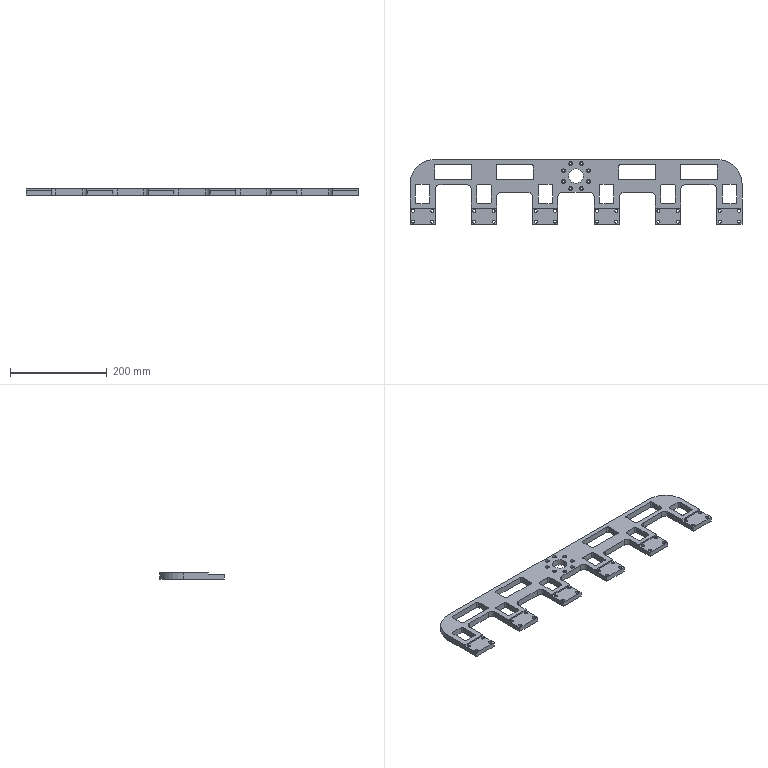NC program | NX | posted with a generic post | part box 687 x 134 x 13 mm
Lines 123 to 1308 of 9954:
(ZLEVEL_PROFILE_COPY_3 , TOOL : D10)
N226 T10 M6
N228 G54
N230 G17 G0 G90 X-335.468 Y52.717 S9500 M3
N232 G43 Z30. H10
N234 Z1.5
N236 G94 G1 X-335.432 Y52.76 Z1.497 F1000.
N238 X-333.485 Y54.925 Z1.344
N240 X-331.425 Y56.985 Z1.192
N242 X-329.26 Y58.932 Z1.039
N244 X-326.995 Y60.763 Z0.887
N246 X-324.636 Y62.471 Z0.734
N248 X-322.191 Y64.053 Z0.581
N250 X-319.665 Y65.503 Z0.429
N252 X-317.066 Y66.817 Z0.276
N254 X-314.402 Y67.992 Z0.123
N256 X-311.679 Y69.025 Z-0.029
N258 X-308.905 Y69.913 Z-0.182
N260 X-306.088 Y70.653 Z-0.334
N262 X-303.236 Y71.243 Z-0.487
N264 X-300.357 Y71.682 Z-0.64
N266 X-297.459 Y71.968 Z-0.792
N268 X-294.55 Y72.1 Z-0.945
N270 X-293.5 Z-1.
N272 X293.5 F3500.
N274 G2 X348.6 Y17. R55.1
N276 G1 Y-67.
N278 G2 X343.5 Y-72.1 R5.1
N280 G1 X291.5
N282 G2 X286.4 Y-67. R5.1
N284 G1 Y5.
N286 G3 X281.5 Y9.9 R4.9
N288 G1 X226.503
N290 G3 X221.6 Y5. R4.9
N292 G1 Y-67.
N294 G2 X216.5 Y-72.1 R5.1
N296 G1 X164.5
N298 G2 X159.4 Y-67. R5.1
N300 G1 Y-10.95
N302 G3 X154.5 Y-6.05 R4.9
N304 G1 X99.5
N306 G3 X94.6 Y-10.95 R4.9
N308 G1 Y-67.
N310 G2 X89.5 Y-72.1 R5.1
N312 G1 X37.5
N314 G2 X32.4 Y-67. R5.1
N316 G1 Y-10.95
N318 G3 X27.5 Y-6.05 R4.9
N320 G1 X-27.499
N322 G3 X-32.4 Y-10.95 R4.9
N324 G1 Y-67.
N326 G2 X-37.5 Y-72.1 R5.1
N328 G1 X-89.5
N330 G2 X-94.6 Y-67. R5.1
N332 G1 Y-10.95
N334 G3 X-99.5 Y-6.05 R4.9
N336 G1 X-154.497
N338 G3 X-159.4 Y-10.95 R4.9
N340 G1 Y-67.
N342 G2 X-164.5 Y-72.1 R5.1
N344 G1 X-216.5
N346 G2 X-221.6 Y-67. R5.1
N348 G1 Y5.
N350 G3 X-226.5 Y9.9 R4.9
N352 G1 X-281.497
N354 G3 X-286.4 Y5. R4.9
N356 G1 Y-67.
N358 G2 X-291.5 Y-72.1 R5.1
N360 G1 X-343.5
N362 G2 X-348.6 Y-67. R5.1
N364 G1 Y17.
N366 G2 X-293.5 Y72.1 R55.1
N368 G1 X-236.21 Z-2.
N370 X293.5
N372 G2 X348.6 Y17. R55.1
N374 G1 Y-67.
N376 G2 X343.5 Y-72.1 R5.1
N378 G1 X291.5
N380 G2 X286.4 Y-67. R5.1
N382 G1 Y5.
N384 G3 X281.5 Y9.9 R4.9
N386 G1 X226.503
N388 G3 X221.6 Y5. R4.9
N390 G1 Y-67.
N392 G2 X216.5 Y-72.1 R5.1
N394 G1 X164.5
N396 G2 X159.4 Y-67. R5.1
N398 G1 Y-10.95
N400 G3 X154.5 Y-6.05 R4.9
N402 G1 X99.5
N404 G3 X94.6 Y-10.95 R4.9
N406 G1 Y-67.
N408 G2 X89.5 Y-72.1 R5.1
N410 G1 X37.5
N412 G2 X32.4 Y-67. R5.1
N414 G1 Y-10.95
N416 G3 X27.5 Y-6.05 R4.9
N418 G1 X-27.499
N420 G3 X-32.4 Y-10.95 R4.9
N422 G1 Y-67.
N424 G2 X-37.5 Y-72.1 R5.1
N426 G1 X-89.5
N428 G2 X-94.6 Y-67. R5.1
N430 G1 Y-10.95
N432 G3 X-99.5 Y-6.05 R4.9
N434 G1 X-154.497
N436 G3 X-159.4 Y-10.95 R4.9
N438 G1 Y-67.
N440 G2 X-164.5 Y-72.1 R5.1
N442 G1 X-216.5
N444 G2 X-221.6 Y-67. R5.1
N446 G1 Y5.
N448 G3 X-226.5 Y9.9 R4.9
N450 G1 X-281.497
N452 G3 X-286.4 Y5. R4.9
N454 G1 Y-67.
N456 G2 X-291.5 Y-72.1 R5.1
N458 G1 X-343.5
N460 G2 X-348.6 Y-67. R5.1
N462 G1 Y17.
N464 G2 X-293.5 Y72.1 R55.1
N466 G1 X-236.21 Z-3.
N468 X293.5
N470 G2 X348.6 Y17. R55.1
N472 G1 Y-67.
N474 G2 X343.5 Y-72.1 R5.1
N476 G1 X291.5
N478 G2 X286.4 Y-67. R5.1
N480 G1 Y5.
N482 G3 X281.5 Y9.9 R4.9
N484 G1 X226.503
N486 G3 X221.6 Y5. R4.9
N488 G1 Y-67.
N490 G2 X216.5 Y-72.1 R5.1
N492 G1 X164.5
N494 G2 X159.4 Y-67. R5.1
N496 G1 Y-10.95
N498 G3 X154.5 Y-6.05 R4.9
N500 G1 X99.5
N502 G3 X94.6 Y-10.95 R4.9
N504 G1 Y-67.
N506 G2 X89.5 Y-72.1 R5.1
N508 G1 X37.5
N510 G2 X32.4 Y-67. R5.1
N512 G1 Y-10.95
N514 G3 X27.5 Y-6.05 R4.9
N516 G1 X-27.499
N518 G3 X-32.4 Y-10.95 R4.9
N520 G1 Y-67.
N522 G2 X-37.5 Y-72.1 R5.1
N524 G1 X-89.5
N526 G2 X-94.6 Y-67. R5.1
N528 G1 Y-10.95
N530 G3 X-99.5 Y-6.05 R4.9
N532 G1 X-154.497
N534 G3 X-159.4 Y-10.95 R4.9
N536 G1 Y-67.
N538 G2 X-164.5 Y-72.1 R5.1
N540 G1 X-216.5
N542 G2 X-221.6 Y-67. R5.1
N544 G1 Y5.
N546 G3 X-226.5 Y9.9 R4.9
N548 G1 X-281.497
N550 G3 X-286.4 Y5. R4.9
N552 G1 Y-67.
N554 G2 X-291.5 Y-72.1 R5.1
N556 G1 X-343.5
N558 G2 X-348.6 Y-67. R5.1
N560 G1 Y17.
N562 G2 X-293.5 Y72.1 R55.1
N564 G1 X-236.21 Z-4.
N566 X293.5
N568 G2 X348.6 Y17. R55.1
N570 G1 Y-67.
N572 G2 X343.5 Y-72.1 R5.1
N574 G1 X291.5
N576 G2 X286.4 Y-67. R5.1
N578 G1 Y5.
N580 G3 X281.5 Y9.9 R4.9
N582 G1 X226.503
N584 G3 X221.6 Y5. R4.9
N586 G1 Y-67.
N588 G2 X216.5 Y-72.1 R5.1
N590 G1 X164.5
N592 G2 X159.4 Y-67. R5.1
N594 G1 Y-10.95
N596 G3 X154.5 Y-6.05 R4.9
N598 G1 X99.5
N600 G3 X94.6 Y-10.95 R4.9
N602 G1 Y-67.
N604 G2 X89.5 Y-72.1 R5.1
N606 G1 X37.5
N608 G2 X32.4 Y-67. R5.1
N610 G1 Y-10.95
N612 G3 X27.5 Y-6.05 R4.9
N614 G1 X-27.499
N616 G3 X-32.4 Y-10.95 R4.9
N618 G1 Y-67.
N620 G2 X-37.5 Y-72.1 R5.1
N622 G1 X-89.5
N624 G2 X-94.6 Y-67. R5.1
N626 G1 Y-10.95
N628 G3 X-99.5 Y-6.05 R4.9
N630 G1 X-154.497
N632 G3 X-159.4 Y-10.95 R4.9
N634 G1 Y-67.
N636 G2 X-164.5 Y-72.1 R5.1
N638 G1 X-216.5
N640 G2 X-221.6 Y-67. R5.1
N642 G1 Y5.
N644 G3 X-226.5 Y9.9 R4.9
N646 G1 X-281.497
N648 G3 X-286.4 Y5. R4.9
N650 G1 Y-67.
N652 G2 X-291.5 Y-72.1 R5.1
N654 G1 X-343.5
N656 G2 X-348.6 Y-67. R5.1
N658 G1 Y17.
N660 G2 X-293.5 Y72.1 R55.1
N662 G1 X-236.21 Z-5.
N664 X293.5
N666 G2 X348.6 Y17. R55.1
N668 G1 Y-67.
N670 G2 X343.5 Y-72.1 R5.1
N672 G1 X291.5
N674 G2 X286.4 Y-67. R5.1
N676 G1 Y5.
N678 G3 X281.5 Y9.9 R4.9
N680 G1 X226.503
N682 G3 X221.6 Y5. R4.9
N684 G1 Y-67.
N686 G2 X216.5 Y-72.1 R5.1
N688 G1 X164.5
N690 G2 X159.4 Y-67. R5.1
N692 G1 Y-10.95
N694 G3 X154.5 Y-6.05 R4.9
N696 G1 X99.5
N698 G3 X94.6 Y-10.95 R4.9
N700 G1 Y-67.
N702 G2 X89.5 Y-72.1 R5.1
N704 G1 X37.5
N706 G2 X32.4 Y-67. R5.1
N708 G1 Y-10.95
N710 G3 X27.5 Y-6.05 R4.9
N712 G1 X-27.499
N714 G3 X-32.4 Y-10.95 R4.9
N716 G1 Y-67.
N718 G2 X-37.5 Y-72.1 R5.1
N720 G1 X-89.5
N722 G2 X-94.6 Y-67. R5.1
N724 G1 Y-10.95
N726 G3 X-99.5 Y-6.05 R4.9
N728 G1 X-154.497
N730 G3 X-159.4 Y-10.95 R4.9
N732 G1 Y-67.
N734 G2 X-164.5 Y-72.1 R5.1
N736 G1 X-216.5
N738 G2 X-221.6 Y-67. R5.1
N740 G1 Y5.
N742 G3 X-226.5 Y9.9 R4.9
N744 G1 X-281.497
N746 G3 X-286.4 Y5. R4.9
N748 G1 Y-67.
N750 G2 X-291.5 Y-72.1 R5.1
N752 G1 X-343.5
N754 G2 X-348.6 Y-67. R5.1
N756 G1 Y17.
N758 G2 X-293.5 Y72.1 R55.1
N760 G1 X-236.21 Z-6.
N762 X293.5
N764 G2 X348.6 Y17. R55.1
N766 G1 Y-67.
N768 G2 X343.5 Y-72.1 R5.1
N770 G1 X291.5
N772 G2 X286.4 Y-67. R5.1
N774 G1 Y5.
N776 G3 X281.5 Y9.9 R4.9
N778 G1 X226.503
N780 G3 X221.6 Y5. R4.9
N782 G1 Y-67.
N784 G2 X216.5 Y-72.1 R5.1
N786 G1 X164.5
N788 G2 X159.4 Y-67. R5.1
N790 G1 Y-10.95
N792 G3 X154.5 Y-6.05 R4.9
N794 G1 X99.5
N796 G3 X94.6 Y-10.95 R4.9
N798 G1 Y-67.
N800 G2 X89.5 Y-72.1 R5.1
N802 G1 X37.5
N804 G2 X32.4 Y-67. R5.1
N806 G1 Y-10.95
N808 G3 X27.5 Y-6.05 R4.9
N810 G1 X-27.499
N812 G3 X-32.4 Y-10.95 R4.9
N814 G1 Y-67.
N816 G2 X-37.5 Y-72.1 R5.1
N818 G1 X-89.5
N820 G2 X-94.6 Y-67. R5.1
N822 G1 Y-10.95
N824 G3 X-99.5 Y-6.05 R4.9
N826 G1 X-154.497
N828 G3 X-159.4 Y-10.95 R4.9
N830 G1 Y-67.
N832 G2 X-164.5 Y-72.1 R5.1
N834 G1 X-216.5
N836 G2 X-221.6 Y-67. R5.1
N838 G1 Y5.
N840 G3 X-226.5 Y9.9 R4.9
N842 G1 X-281.497
N844 G3 X-286.4 Y5. R4.9
N846 G1 Y-67.
N848 G2 X-291.5 Y-72.1 R5.1
N850 G1 X-343.5
N852 G2 X-348.6 Y-67. R5.1
N854 G1 Y17.
N856 G2 X-293.5 Y72.1 R55.1
N858 G1 X-236.21 Z-7.
N860 X293.5
N862 G2 X348.6 Y17. R55.1
N864 G1 Y-67.
N866 G2 X343.5 Y-72.1 R5.1
N868 G1 X291.5
N870 G2 X286.4 Y-67. R5.1
N872 G1 Y5.
N874 G3 X281.5 Y9.9 R4.9
N876 G1 X226.503
N878 G3 X221.6 Y5. R4.9
N880 G1 Y-67.
N882 G2 X216.5 Y-72.1 R5.1
N884 G1 X164.5
N886 G2 X159.4 Y-67. R5.1
N888 G1 Y-10.95
N890 G3 X154.5 Y-6.05 R4.9
N892 G1 X99.5
N894 G3 X94.6 Y-10.95 R4.9
N896 G1 Y-67.
N898 G2 X89.5 Y-72.1 R5.1
N900 G1 X37.5
N902 G2 X32.4 Y-67. R5.1
N904 G1 Y-10.95
N906 G3 X27.5 Y-6.05 R4.9
N908 G1 X-27.499
N910 G3 X-32.4 Y-10.95 R4.9
N912 G1 Y-67.
N914 G2 X-37.5 Y-72.1 R5.1
N916 G1 X-89.5
N918 G2 X-94.6 Y-67. R5.1
N920 G1 Y-10.95
N922 G3 X-99.5 Y-6.05 R4.9
N924 G1 X-154.497
N926 G3 X-159.4 Y-10.95 R4.9
N928 G1 Y-67.
N930 G2 X-164.5 Y-72.1 R5.1
N932 G1 X-216.5
N934 G2 X-221.6 Y-67. R5.1
N936 G1 Y5.
N938 G3 X-226.5 Y9.9 R4.9
N940 G1 X-281.497
N942 G3 X-286.4 Y5. R4.9
N944 G1 Y-67.
N946 G2 X-291.5 Y-72.1 R5.1
N948 G1 X-343.5
N950 G2 X-348.6 Y-67. R5.1
N952 G1 Y17.
N954 G2 X-293.5 Y72.1 R55.1
N956 G1 X-236.21 Z-8.
N958 X293.5
N960 G2 X348.6 Y17. R55.1
N962 G1 Y-67.
N964 G2 X343.5 Y-72.1 R5.1
N966 G1 X291.5
N968 G2 X286.4 Y-67. R5.1
N970 G1 Y5.
N972 G3 X281.5 Y9.9 R4.9
N974 G1 X226.503
N976 G3 X221.6 Y5. R4.9
N978 G1 Y-67.
N980 G2 X216.5 Y-72.1 R5.1
N982 G1 X164.5
N984 G2 X159.4 Y-67. R5.1
N986 G1 Y-10.95
N988 G3 X154.5 Y-6.05 R4.9
N990 G1 X99.5
N992 G3 X94.6 Y-10.95 R4.9
N994 G1 Y-67.
N996 G2 X89.5 Y-72.1 R5.1
N998 G1 X37.5
N1000 G2 X32.4 Y-67. R5.1
N1002 G1 Y-10.95
N1004 G3 X27.5 Y-6.05 R4.9
N1006 G1 X-27.499
N1008 G3 X-32.4 Y-10.95 R4.9
N1010 G1 Y-67.
N1012 G2 X-37.5 Y-72.1 R5.1
N1014 G1 X-89.5
N1016 G2 X-94.6 Y-67. R5.1
N1018 G1 Y-10.95
N1020 G3 X-99.5 Y-6.05 R4.9
N1022 G1 X-154.497
N1024 G3 X-159.4 Y-10.95 R4.9
N1026 G1 Y-67.
N1028 G2 X-164.5 Y-72.1 R5.1
N1030 G1 X-216.5
N1032 G2 X-221.6 Y-67. R5.1
N1034 G1 Y5.
N1036 G3 X-226.5 Y9.9 R4.9
N1038 G1 X-281.497
N1040 G3 X-286.4 Y5. R4.9
N1042 G1 Y-67.
N1044 G2 X-291.5 Y-72.1 R5.1
N1046 G1 X-343.5
N1048 G2 X-348.6 Y-67. R5.1
N1050 G1 Y17.
N1052 G2 X-293.5 Y72.1 R55.1
N1054 G1 X-236.21 Z-9.
N1056 X293.5
N1058 G2 X348.6 Y17. R55.1
N1060 G1 Y-67.
N1062 G2 X343.5 Y-72.1 R5.1
N1064 G1 X291.5
N1066 G2 X286.4 Y-67. R5.1
N1068 G1 Y5.
N1070 G3 X281.5 Y9.9 R4.9
N1072 G1 X226.503
N1074 G3 X221.6 Y5. R4.9
N1076 G1 Y-67.
N1078 G2 X216.5 Y-72.1 R5.1
N1080 G1 X164.5
N1082 G2 X159.4 Y-67. R5.1
N1084 G1 Y-10.95
N1086 G3 X154.5 Y-6.05 R4.9
N1088 G1 X99.5
N1090 G3 X94.6 Y-10.95 R4.9
N1092 G1 Y-67.
N1094 G2 X89.5 Y-72.1 R5.1
N1096 G1 X37.5
N1098 G2 X32.4 Y-67. R5.1
N1100 G1 Y-10.95
N1102 G3 X27.5 Y-6.05 R4.9
N1104 G1 X-27.499
N1106 G3 X-32.4 Y-10.95 R4.9
N1108 G1 Y-67.
N1110 G2 X-37.5 Y-72.1 R5.1
N1112 G1 X-89.5
N1114 G2 X-94.6 Y-67. R5.1
N1116 G1 Y-10.95
N1118 G3 X-99.5 Y-6.05 R4.9
N1120 G1 X-154.497
N1122 G3 X-159.4 Y-10.95 R4.9
N1124 G1 Y-67.
N1126 G2 X-164.5 Y-72.1 R5.1
N1128 G1 X-216.5
N1130 G2 X-221.6 Y-67. R5.1
N1132 G1 Y5.
N1134 G3 X-226.5 Y9.9 R4.9
N1136 G1 X-281.497
N1138 G3 X-286.4 Y5. R4.9
N1140 G1 Y-67.
N1142 G2 X-291.5 Y-72.1 R5.1
N1144 G1 X-343.5
N1146 G2 X-348.6 Y-67. R5.1
N1148 G1 Y17.
N1150 G2 X-293.5 Y72.1 R55.1
N1152 G1 X-236.21 Z-10.
N1154 X293.5
N1156 G2 X348.6 Y17. R55.1
N1158 G1 Y-67.
N1160 G2 X343.5 Y-72.1 R5.1
N1162 G1 X291.5
N1164 G2 X286.4 Y-67. R5.1
N1166 G1 Y5.
N1168 G3 X281.5 Y9.9 R4.9
N1170 G1 X226.503
N1172 G3 X221.6 Y5. R4.9
N1174 G1 Y-67.
N1176 G2 X216.5 Y-72.1 R5.1
N1178 G1 X164.5
N1180 G2 X159.4 Y-67. R5.1
N1182 G1 Y-10.95
N1184 G3 X154.5 Y-6.05 R4.9
N1186 G1 X99.5
N1188 G3 X94.6 Y-10.95 R4.9
N1190 G1 Y-67.
N1192 G2 X89.5 Y-72.1 R5.1
N1194 G1 X37.5
N1196 G2 X32.4 Y-67. R5.1
N1198 G1 Y-10.95
N1200 G3 X27.5 Y-6.05 R4.9
N1202 G1 X-27.499
N1204 G3 X-32.4 Y-10.95 R4.9
N1206 G1 Y-67.
N1208 G2 X-37.5 Y-72.1 R5.1
N1210 G1 X-89.5
N1212 G2 X-94.6 Y-67. R5.1
N1214 G1 Y-10.95
N1216 G3 X-99.5 Y-6.05 R4.9
N1218 G1 X-154.497
N1220 G3 X-159.4 Y-10.95 R4.9
N1222 G1 Y-67.
N1224 G2 X-164.5 Y-72.1 R5.1
N1226 G1 X-216.5
N1228 G2 X-221.6 Y-67. R5.1
N1230 G1 Y5.
N1232 G3 X-226.5 Y9.9 R4.9
N1234 G1 X-281.497
N1236 G3 X-286.4 Y5. R4.9
N1238 G1 Y-67.
N1240 G2 X-291.5 Y-72.1 R5.1
N1242 G1 X-343.5
N1244 G2 X-348.6 Y-67. R5.1
N1246 G1 Y17.
N1248 G2 X-293.5 Y72.1 R55.1
N1250 G1 X-236.21 Z-11.
N1252 X293.5
N1254 G2 X348.6 Y17. R55.1
N1256 G1 Y-67.
N1258 G2 X343.5 Y-72.1 R5.1
N1260 G1 X291.5
N1262 G2 X286.4 Y-67. R5.1
N1264 G1 Y5.
N1266 G3 X281.5 Y9.9 R4.9
N1268 G1 X226.503
N1270 G3 X221.6 Y5. R4.9
N1272 G1 Y-67.
N1274 G2 X216.5 Y-72.1 R5.1
N1276 G1 X164.5
N1278 G2 X159.4 Y-67. R5.1
N1280 G1 Y-10.95
N1282 G3 X154.5 Y-6.05 R4.9
N1284 G1 X99.5
N1286 G3 X94.6 Y-10.95 R4.9
N1288 G1 Y-67.
N1290 G2 X89.5 Y-72.1 R5.1
N1292 G1 X37.5
N1294 G2 X32.4 Y-67. R5.1
N1296 G1 Y-10.95
N1298 G3 X27.5 Y-6.05 R4.9
N1300 G1 X-27.499
N1302 G3 X-32.4 Y-10.95 R4.9
N1304 G1 Y-67.
N1306 G2 X-37.5 Y-72.1 R5.1
N1308 G1 X-89.5
N1310 G2 X-94.6 Y-67. R5.1
N1312 G1 Y-10.95
N1314 G3 X-99.5 Y-6.05 R4.9
N1316 G1 X-154.497
N1318 G3 X-159.4 Y-10.95 R4.9
N1320 G1 Y-67.
N1322 G2 X-164.5 Y-72.1 R5.1
N1324 G1 X-216.5
N1326 G2 X-221.6 Y-67. R5.1
N1328 G1 Y5.
N1330 G3 X-226.5 Y9.9 R4.9
N1332 G1 X-281.497
N1334 G3 X-286.4 Y5. R4.9
N1336 G1 Y-67.
N1338 G2 X-291.5 Y-72.1 R5.1
N1340 G1 X-343.5
N1342 G2 X-348.6 Y-67. R5.1
N1344 G1 Y17.
N1346 G2 X-293.5 Y72.1 R55.1
N1348 G1 X-236.21 Z-12.
N1350 X293.5
N1352 G2 X348.6 Y17. R55.1
N1354 G1 Y-67.
N1356 G2 X343.5 Y-72.1 R5.1
N1358 G1 X291.5
N1360 G2 X286.4 Y-67. R5.1
N1362 G1 Y5.
N1364 G3 X281.5 Y9.9 R4.9
N1366 G1 X226.503
N1368 G3 X221.6 Y5. R4.9
N1370 G1 Y-67.
N1372 G2 X216.5 Y-72.1 R5.1
N1374 G1 X164.5
N1376 G2 X159.4 Y-67. R5.1
N1378 G1 Y-10.95
N1380 G3 X154.5 Y-6.05 R4.9
N1382 G1 X99.5
N1384 G3 X94.6 Y-10.95 R4.9
N1386 G1 Y-67.
N1388 G2 X89.5 Y-72.1 R5.1
N1390 G1 X37.5
N1392 G2 X32.4 Y-67. R5.1
N1394 G1 Y-10.95
N1396 G3 X27.5 Y-6.05 R4.9
N1398 G1 X-27.499
N1400 G3 X-32.4 Y-10.95 R4.9
N1402 G1 Y-67.
N1404 G2 X-37.5 Y-72.1 R5.1
N1406 G1 X-89.5
N1408 G2 X-94.6 Y-67. R5.1
N1410 G1 Y-10.95
N1412 G3 X-99.5 Y-6.05 R4.9
N1414 G1 X-154.497
N1416 G3 X-159.4 Y-10.95 R4.9
N1418 G1 Y-67.
N1420 G2 X-164.5 Y-72.1 R5.1
N1422 G1 X-216.5
N1424 G2 X-221.6 Y-67. R5.1
N1426 G1 Y5.
N1428 G3 X-226.5 Y9.9 R4.9
N1430 G1 X-281.497
N1432 G3 X-286.4 Y5. R4.9
N1434 G1 Y-67.
N1436 G2 X-291.5 Y-72.1 R5.1
N1438 G1 X-343.5
N1440 G2 X-348.6 Y-67. R5.1
N1442 G1 Y17.
N1444 G2 X-293.5 Y72.1 R55.1
N1446 G1 X-236.21 Z-13.
N1448 X293.5
N1450 G2 X348.6 Y17. R55.1
N1452 G1 Y-67.
N1454 G2 X343.5 Y-72.1 R5.1
N1456 G1 X291.5
N1458 G2 X286.4 Y-67. R5.1
N1460 G1 Y5.
N1462 G3 X281.5 Y9.9 R4.9
N1464 G1 X226.503
N1466 G3 X221.6 Y5. R4.9
N1468 G1 Y-67.
N1470 G2 X216.5 Y-72.1 R5.1
N1472 G1 X164.5
N1474 G2 X159.4 Y-67. R5.1
N1476 G1 Y-10.95
N1478 G3 X154.5 Y-6.05 R4.9
N1480 G1 X99.5
N1482 G3 X94.6 Y-10.95 R4.9
N1484 G1 Y-67.
N1486 G2 X89.5 Y-72.1 R5.1
N1488 G1 X37.5
N1490 G2 X32.4 Y-67. R5.1
N1492 G1 Y-10.95
N1494 G3 X27.5 Y-6.05 R4.9
N1496 G1 X-27.499
N1498 G3 X-32.4 Y-10.95 R4.9
N1500 G1 Y-67.
N1502 G2 X-37.5 Y-72.1 R5.1
N1504 G1 X-89.5
N1506 G2 X-94.6 Y-67. R5.1
N1508 G1 Y-10.95
N1510 G3 X-99.5 Y-6.05 R4.9
N1512 G1 X-154.497
N1514 G3 X-159.4 Y-10.95 R4.9
N1516 G1 Y-67.
N1518 G2 X-164.5 Y-72.1 R5.1
N1520 G1 X-216.5
N1522 G2 X-221.6 Y-67. R5.1
N1524 G1 Y5.
N1526 G3 X-226.5 Y9.9 R4.9
N1528 G1 X-281.497
N1530 G3 X-286.4 Y5. R4.9
N1532 G1 Y-67.
N1534 G2 X-291.5 Y-72.1 R5.1
N1536 G1 X-343.5
N1538 G2 X-348.6 Y-67. R5.1
N1540 G1 Y17.
N1542 G2 X-293.5 Y72.1 R55.1
N1544 G1 X-236.21 Z-14.
N1546 X293.5
N1548 G2 X348.6 Y17. R55.1
N1550 G1 Y-67.
N1552 G2 X343.5 Y-72.1 R5.1
N1554 G1 X291.5
N1556 G2 X286.4 Y-67. R5.1
N1558 G1 Y5.
N1560 G3 X281.5 Y9.9 R4.9
N1562 G1 X226.503
N1564 G3 X221.6 Y5. R4.9
N1566 G1 Y-67.
N1568 G2 X216.5 Y-72.1 R5.1
N1570 G1 X164.5
N1572 G2 X159.4 Y-67. R5.1
N1574 G1 Y-10.95
N1576 G3 X154.5 Y-6.05 R4.9
N1578 G1 X99.5
N1580 G3 X94.6 Y-10.95 R4.9
N1582 G1 Y-67.
N1584 G2 X89.5 Y-72.1 R5.1
N1586 G1 X37.5
N1588 G2 X32.4 Y-67. R5.1
N1590 G1 Y-10.95
N1592 G3 X27.5 Y-6.05 R4.9
N1594 G1 X-27.499
N1596 G3 X-32.4 Y-10.95 R4.9
N1598 G1 Y-67.
N1600 G2 X-37.5 Y-72.1 R5.1
N1602 G1 X-89.5
N1604 G2 X-94.6 Y-67. R5.1
N1606 G1 Y-10.95
N1608 G3 X-99.5 Y-6.05 R4.9
N1610 G1 X-154.497
N1612 G3 X-159.4 Y-10.95 R4.9
N1614 G1 Y-67.
N1616 G2 X-164.5 Y-72.1 R5.1
N1618 G1 X-216.5
N1620 G2 X-221.6 Y-67. R5.1
N1622 G1 Y5.
N1624 G3 X-226.5 Y9.9 R4.9
N1626 G1 X-281.497
N1628 G3 X-286.4 Y5. R4.9
N1630 G1 Y-67.
N1632 G2 X-291.5 Y-72.1 R5.1
N1634 G1 X-343.5
N1636 G2 X-348.6 Y-67. R5.1
N1638 G1 Y17.
N1640 G2 X-293.5 Y72.1 R55.1
N1642 G1 X-236.21
N1644 Z-12.5
N1646 G0 Z30.
(ZLEVEL_PROFILE_COPY_2_COPY_COPY , TOOL : D10)
N1648 X148.981 Y35.
N1650 Z1.5
N1652 G1 X155.5 Z1.158 F1000.
N1654 Y47.002 Z0.529
N1656 X155.447 Y47. Z0.527
N1658 X127. Z-0.964
N1660 X98.538 F2000.
N1662 X98.5 Y47.002
N1664 Y35.
N1666 X155.5
N1668 Y47.002
N1670 X155.447 Y47.
N1672 X127.
N1674 X98.75 Z-1.457
N1676 X98.5 Z-1.462
N1678 Y46.625 Z-1.468
N1680 Y35. Z-1.671
N1682 X113.241 Z-1.929
N1684 X155.5
N1686 Y47.002
N1688 X155.447 Y47.
N1690 X127.
N1692 X98.75 Z-2.422
N1694 X98.5 Z-2.426
N1696 Y46.625 Z-2.433
N1698 Y35. Z-2.636
N1700 X113.241 Z-2.893
N1702 X155.5
N1704 Y47.002
N1706 X155.447 Y47.
N1708 X127.
N1710 X98.75 Z-3.386
N1712 X98.5 Z-3.39
N1714 Y46.625 Z-3.397
N1716 Y35. Z-3.6
N1718 X113.241 Z-3.857
N1720 X155.5
N1722 Y47.002
N1724 X155.447 Y47.
N1726 X127.
N1728 X98.75 Z-4.35
N1730 X98.5 Z-4.355
N1732 Y46.625 Z-4.361
N1734 Y35. Z-4.564
N1736 X113.241 Z-4.821
N1738 X155.5
N1740 Y47.002
N1742 X155.447 Y47.
N1744 X127.
N1746 X98.75 Z-5.315
N1748 X98.5 Z-5.319
N1750 Y46.625 Z-5.325
N1752 Y35. Z-5.528
N1754 X113.241 Z-5.786
N1756 X155.5
N1758 Y47.002
N1760 X155.447 Y47.
N1762 X127.
N1764 X98.75 Z-6.279
N1766 X98.5 Z-6.283
N1768 Y46.625 Z-6.29
N1770 Y35. Z-6.493
N1772 X113.241 Z-6.75
N1774 X155.5
N1776 Y47.002
N1778 X155.447 Y47.
N1780 X127.
N1782 X98.75 Z-7.243
N1784 X98.5 Z-7.247
N1786 Y46.625 Z-7.254
N1788 Y35. Z-7.457
N1790 X113.241 Z-7.714
N1792 X155.5
N1794 Y47.002
N1796 X155.447 Y47.
N1798 X127.
N1800 X98.75 Z-8.207
N1802 X98.5 Z-8.212
N1804 Y46.625 Z-8.218
N1806 Y35. Z-8.421
N1808 X113.241 Z-8.679
N1810 X155.5
N1812 Y47.002
N1814 X155.447 Y47.
N1816 X127.
N1818 X98.75 Z-9.172
N1820 X98.5 Z-9.176
N1822 Y46.625 Z-9.183
N1824 Y35. Z-9.386
N1826 X113.241 Z-9.643
N1828 X155.5
N1830 Y47.002
N1832 X155.447 Y47.
N1834 X127.
N1836 X98.75 Z-10.136
N1838 X98.5 Z-10.14
N1840 Y46.625 Z-10.147
N1842 Y35. Z-10.35
N1844 X113.241 Z-10.607
N1846 X155.5
N1848 Y47.002
N1850 X155.447 Y47.
N1852 X127.
N1854 X98.75 Z-11.1
N1856 X98.5 Z-11.105
N1858 Y46.625 Z-11.111
N1860 Y35. Z-11.314
N1862 X113.241 Z-11.571
N1864 X155.5
N1866 Y47.002
N1868 X155.447 Y47.
N1870 X127.
N1872 X98.75 Z-12.065
N1874 X98.5 Z-12.069
N1876 Y46.625 Z-12.075
N1878 Y35. Z-12.278
N1880 X113.241 Z-12.536
N1882 X155.5
N1884 Y47.002
N1886 X155.447 Y47.
N1888 X127.
N1890 X98.75 Z-13.029
N1892 X98.5 Z-13.033
N1894 Y46.625 Z-13.04
N1896 Y35. Z-13.243
N1898 X113.241 Z-13.5
N1900 X155.5
N1902 Y47.002
N1904 X155.447 Y47.
N1906 X98.538
N1908 X98.5 Y47.002
N1910 Y35.
N1912 X113.241
N1914 Z-12.
N1916 G0 Z30.
N1918 X-105.019
N1920 Z1.5
N1922 G1 X-98.5 Z1.158 F1000.
N1924 Y47.002 Z0.529
N1926 X-98.538 Y47. Z0.527
N1928 X-127. Z-0.964
N1930 X-155.447 F2000.
N1932 X-155.5 Y47.002
N1934 Y35.
N1936 X-98.5
N1938 Y47.002
N1940 X-98.538 Y47.
N1942 X-127.
N1944 X-155.25 Z-1.457
N1946 X-155.5 Z-1.462
N1948 Y46.625 Z-1.468
N1950 Y35. Z-1.671
N1952 X-140.758 Z-1.929
N1954 X-98.5
N1956 Y47.002
N1958 X-98.538 Y47.
N1960 X-127.
N1962 X-155.25 Z-2.422
N1964 X-155.5 Z-2.426
N1966 Y46.625 Z-2.433
N1968 Y35. Z-2.636
N1970 X-140.758 Z-2.893
N1972 X-98.5
N1974 Y47.002
N1976 X-98.538 Y47.
N1978 X-127.
N1980 X-155.25 Z-3.386
N1982 X-155.5 Z-3.39
N1984 Y46.625 Z-3.397
N1986 Y35. Z-3.6
N1988 X-140.758 Z-3.857
N1990 X-98.5
N1992 Y47.002
N1994 X-98.538 Y47.
N1996 X-127.
N1998 X-155.25 Z-4.35
N2000 X-155.5 Z-4.355
N2002 Y46.625 Z-4.361
N2004 Y35. Z-4.564
N2006 X-140.758 Z-4.821
N2008 X-98.5
N2010 Y47.002
N2012 X-98.538 Y47.
N2014 X-127.
N2016 X-155.25 Z-5.315
N2018 X-155.5 Z-5.319
N2020 Y46.625 Z-5.325
N2022 Y35. Z-5.528
N2024 X-140.758 Z-5.786
N2026 X-98.5
N2028 Y47.002
N2030 X-98.538 Y47.
N2032 X-127.
N2034 X-155.25 Z-6.279
N2036 X-155.5 Z-6.283
N2038 Y46.625 Z-6.29
N2040 Y35. Z-6.493
N2042 X-140.758 Z-6.75
N2044 X-98.5
N2046 Y47.002
N2048 X-98.538 Y47.
N2050 X-127.
N2052 X-155.25 Z-7.243
N2054 X-155.5 Z-7.247
N2056 Y46.625 Z-7.254
N2058 Y35. Z-7.457
N2060 X-140.758 Z-7.714
N2062 X-98.5
N2064 Y47.002
N2066 X-98.538 Y47.
N2068 X-127.
N2070 X-155.25 Z-8.207
N2072 X-155.5 Z-8.212
N2074 Y46.625 Z-8.218
N2076 Y35. Z-8.421
N2078 X-140.758 Z-8.679
N2080 X-98.5
N2082 Y47.002
N2084 X-98.538 Y47.
N2086 X-127.
N2088 X-155.25 Z-9.172
N2090 X-155.5 Z-9.176
N2092 Y46.625 Z-9.183
N2094 Y35. Z-9.386
N2096 X-140.758 Z-9.643
N2098 X-98.5
N2100 Y47.002
N2102 X-98.538 Y47.
N2104 X-127.
N2106 X-155.25 Z-10.136
N2108 X-155.5 Z-10.14
N2110 Y46.625 Z-10.147
N2112 Y35. Z-10.35
N2114 X-140.758 Z-10.607
N2116 X-98.5
N2118 Y47.002
N2120 X-98.538 Y47.
N2122 X-127.
N2124 X-155.25 Z-11.1
N2126 X-155.5 Z-11.105
N2128 Y46.625 Z-11.111
N2130 Y35. Z-11.314
N2132 X-140.758 Z-11.571
N2134 X-98.5
N2136 Y47.002
N2138 X-98.538 Y47.
N2140 X-127.
N2142 X-155.25 Z-12.065
N2144 X-155.5 Z-12.069
N2146 Y46.625 Z-12.075
N2148 Y35. Z-12.278
N2150 X-140.758 Z-12.536
N2152 X-98.5
N2154 Y47.002
N2156 X-98.538 Y47.
N2158 X-127.
N2160 X-155.25 Z-13.029
N2162 X-155.5 Z-13.033
N2164 Y46.625 Z-13.04
N2166 Y35. Z-13.243
N2168 X-140.758 Z-13.5
N2170 X-98.5
N2172 Y47.002
N2174 X-98.538 Y47.
N2176 X-155.447
N2178 X-155.5 Y47.002
N2180 Y35.
N2182 X-140.758
N2184 Z-12.
N2186 G0 Z30.
N2188 X275.981
N2190 Z1.5
N2192 G1 X282.5 Z1.158 F1000.
N2194 Y47.002 Z0.529
N2196 X282.453 Y47. Z0.527
N2198 X254. Z-0.964
N2200 X225.541 F2000.
N2202 X225.5 Y47.002
N2204 Y35.
N2206 X282.5
N2208 Y47.002
N2210 X282.453 Y47.
N2212 X254.
N2214 X225.75 Z-1.457
N2216 X225.5 Z-1.462
N2218 Y46.625 Z-1.468
N2220 Y35. Z-1.671
N2222 X240.242 Z-1.929
N2224 X282.5
N2226 Y47.002
N2228 X282.453 Y47.
N2230 X254.
N2232 X225.75 Z-2.422
N2234 X225.5 Z-2.426
N2236 Y46.625 Z-2.433
N2238 Y35. Z-2.636
N2240 X240.242 Z-2.893
N2242 X282.5
N2244 Y47.002
N2246 X282.453 Y47.
N2248 X254.
N2250 X225.75 Z-3.386
N2252 X225.5 Z-3.39
N2254 Y46.625 Z-3.397
N2256 Y35. Z-3.6
N2258 X240.242 Z-3.857
N2260 X282.5
N2262 Y47.002
N2264 X282.453 Y47.
N2266 X254.
N2268 X225.75 Z-4.35
N2270 X225.5 Z-4.355
N2272 Y46.625 Z-4.361
N2274 Y35. Z-4.564
N2276 X240.242 Z-4.821
N2278 X282.5
N2280 Y47.002
N2282 X282.453 Y47.
N2284 X254.
N2286 X225.75 Z-5.315
N2288 X225.5 Z-5.319
N2290 Y46.625 Z-5.325
N2292 Y35. Z-5.528
N2294 X240.242 Z-5.786
N2296 X282.5
N2298 Y47.002
N2300 X282.453 Y47.
N2302 X254.
N2304 X225.75 Z-6.279
N2306 X225.5 Z-6.283
N2308 Y46.625 Z-6.29
N2310 Y35. Z-6.493
N2312 X240.242 Z-6.75
N2314 X282.5
N2316 Y47.002
N2318 X282.453 Y47.
N2320 X254.
N2322 X225.75 Z-7.243
N2324 X225.5 Z-7.247
N2326 Y46.625 Z-7.254
N2328 Y35. Z-7.457
N2330 X240.242 Z-7.714
N2332 X282.5
N2334 Y47.002
N2336 X282.453 Y47.
N2338 X254.
N2340 X225.75 Z-8.207
N2342 X225.5 Z-8.212
N2344 Y46.625 Z-8.218
N2346 Y35. Z-8.421
N2348 X240.242 Z-8.679
N2350 X282.5
N2352 Y47.002
N2354 X282.453 Y47.
N2356 X254.
N2358 X225.75 Z-9.172
N2360 X225.5 Z-9.176
N2362 Y46.625 Z-9.183
N2364 Y35. Z-9.386
N2366 X240.242 Z-9.643
N2368 X282.5
N2370 Y47.002
N2372 X282.453 Y47.
N2374 X254.
N2376 X225.75 Z-10.136
N2378 X225.5 Z-10.14
N2380 Y46.625 Z-10.147
N2382 Y35. Z-10.35
N2384 X240.242 Z-10.607
N2386 X282.5
N2388 Y47.002
N2390 X282.453 Y47.
N2392 X254.
N2394 X225.75 Z-11.1
N2396 X225.5 Z-11.105
N2398 Y46.625 Z-11.111
N2400 Y35. Z-11.314
N2402 X240.242 Z-11.571
N2404 X282.5
N2406 Y47.002
N2408 X282.453 Y47.
N2410 X254.
N2412 X225.75 Z-12.065
N2414 X225.5 Z-12.069
N2416 Y46.625 Z-12.075
N2418 Y35. Z-12.278
N2420 X240.242 Z-12.536
N2422 X282.5
N2424 Y47.002
N2426 X282.453 Y47.
N2428 X254.
N2430 X225.75 Z-13.029
N2432 X225.5 Z-13.033
N2434 Y46.625 Z-13.04
N2436 Y35. Z-13.243
N2438 X240.242 Z-13.5
N2440 X282.5
N2442 Y47.002
N2444 X282.453 Y47.
N2446 X225.541
N2448 X225.5 Y47.002
N2450 Y35.
N2452 X240.242
N2454 Z-12.
N2456 G0 Z30.
N2458 X-232.019
N2460 Z1.5
N2462 G1 X-225.5 Z1.158 F1000.
N2464 Y47.002 Z0.529
N2466 X-225.541 Y47. Z0.527
N2468 X-254. Z-0.964
N2470 X-282.453 F2000.
N2472 X-282.5 Y47.002
N2474 Y35.
N2476 X-225.5
N2478 Y47.002
N2480 X-225.541 Y47.
N2482 X-254.
N2484 X-282.25 Z-1.457
N2486 X-282.5 Z-1.462
N2488 Y46.625 Z-1.468
N2490 Y35. Z-1.671
N2492 X-267.758 Z-1.929
N2494 X-225.5
N2496 Y47.002
N2498 X-225.541 Y47.
N2500 X-254.
N2502 X-282.25 Z-2.422
N2504 X-282.5 Z-2.426
N2506 Y46.625 Z-2.433
N2508 Y35. Z-2.636
N2510 X-267.758 Z-2.893
N2512 X-225.5
N2514 Y47.002
N2516 X-225.541 Y47.
N2518 X-254.
N2520 X-282.25 Z-3.386
N2522 X-282.5 Z-3.39
N2524 Y46.625 Z-3.397
N2526 Y35. Z-3.6
N2528 X-267.758 Z-3.857
N2530 X-225.5
N2532 Y47.002
N2534 X-225.541 Y47.
N2536 X-254.
N2538 X-282.25 Z-4.35
N2540 X-282.5 Z-4.355
N2542 Y46.625 Z-4.361
N2544 Y35. Z-4.564
N2546 X-267.758 Z-4.821
N2548 X-225.5
N2550 Y47.002
N2552 X-225.541 Y47.
N2554 X-254.
N2556 X-282.25 Z-5.315
N2558 X-282.5 Z-5.319
N2560 Y46.625 Z-5.325
N2562 Y35. Z-5.528
N2564 X-267.758 Z-5.786
N2566 X-225.5
N2568 Y47.002
N2570 X-225.541 Y47.
N2572 X-254.
N2574 X-282.25 Z-6.279
N2576 X-282.5 Z-6.283
N2578 Y46.625 Z-6.29
N2580 Y35. Z-6.493
N2582 X-267.758 Z-6.75
N2584 X-225.5